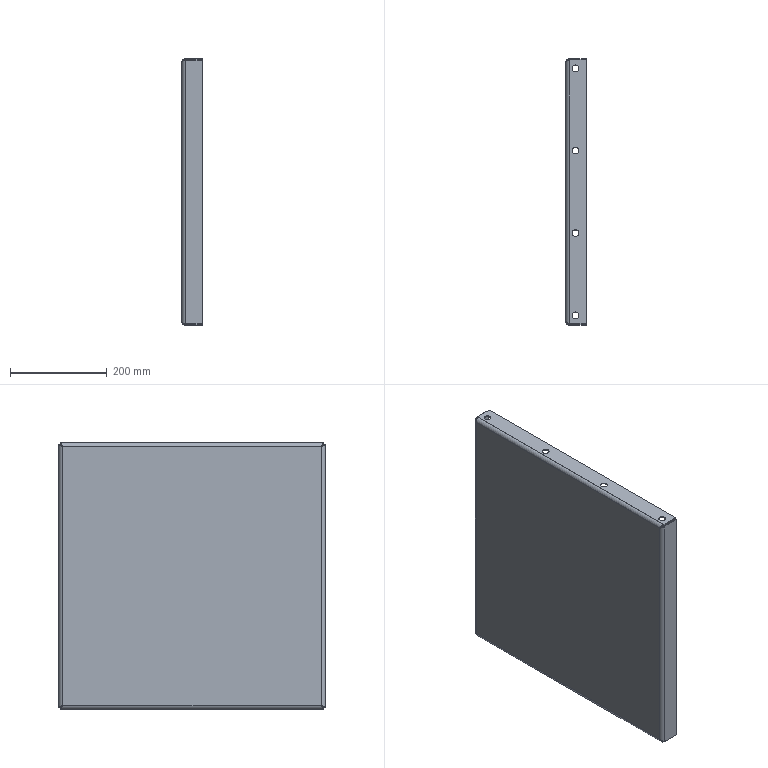Part | STEP file | Produce dryer line heating fan-OVEN-452 | 1 solid | 54 faces | box 42 x 550 x 550 mm | volume 763414 mm3 | cylinder 24 | plane 22 | spline 8 | commonest cylinder face diameters 14 x16 12 x4 16 x4